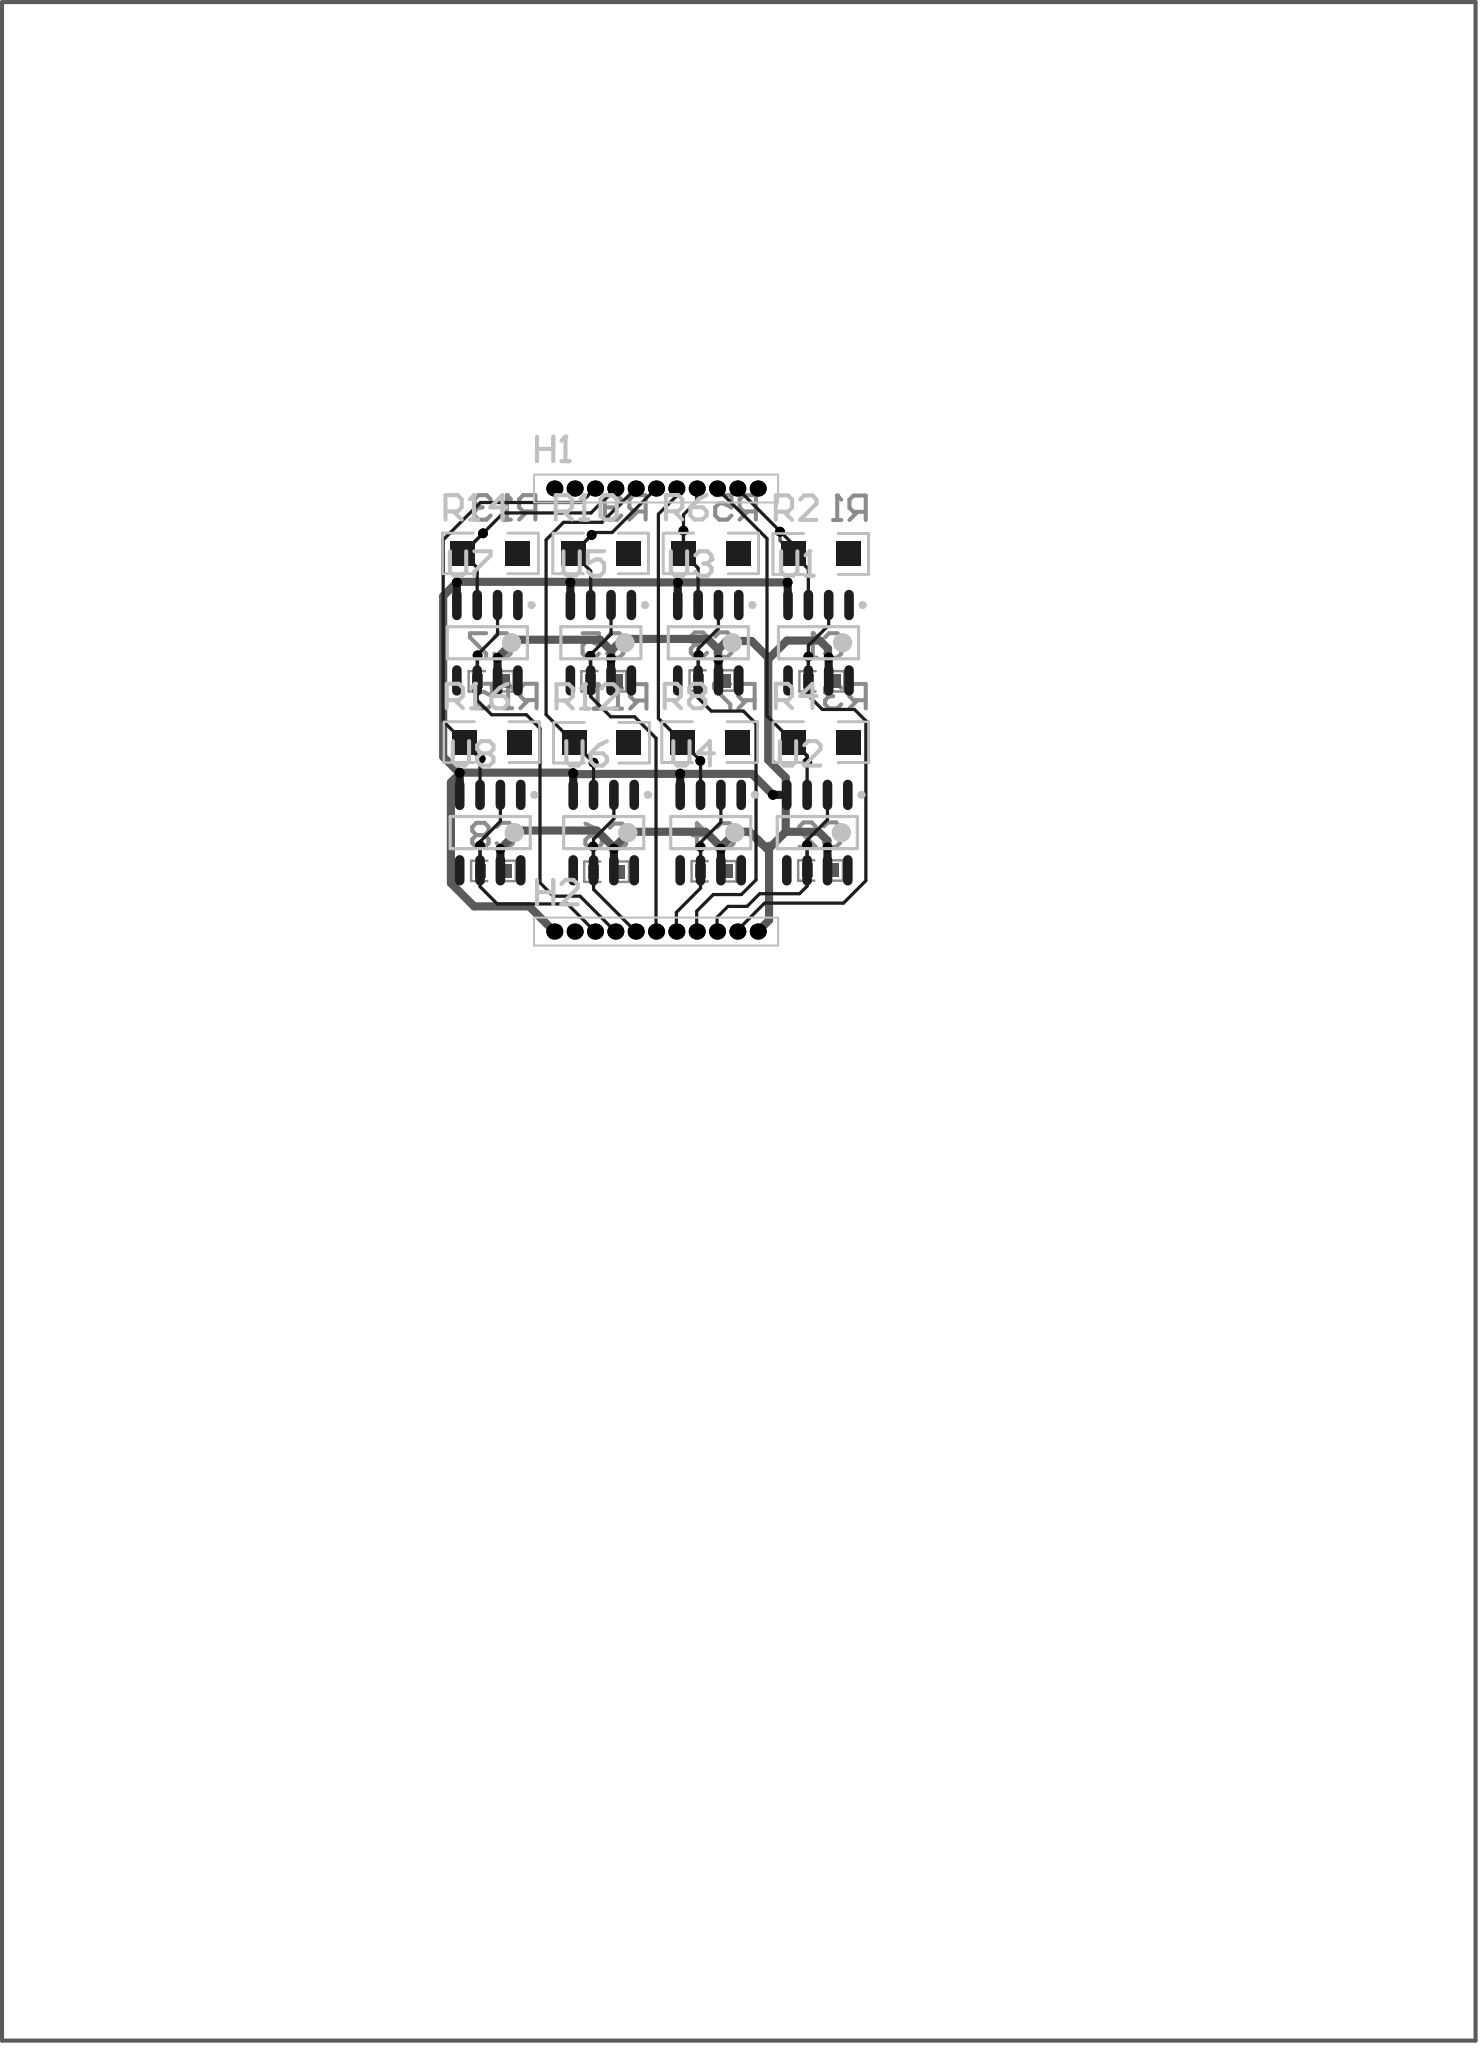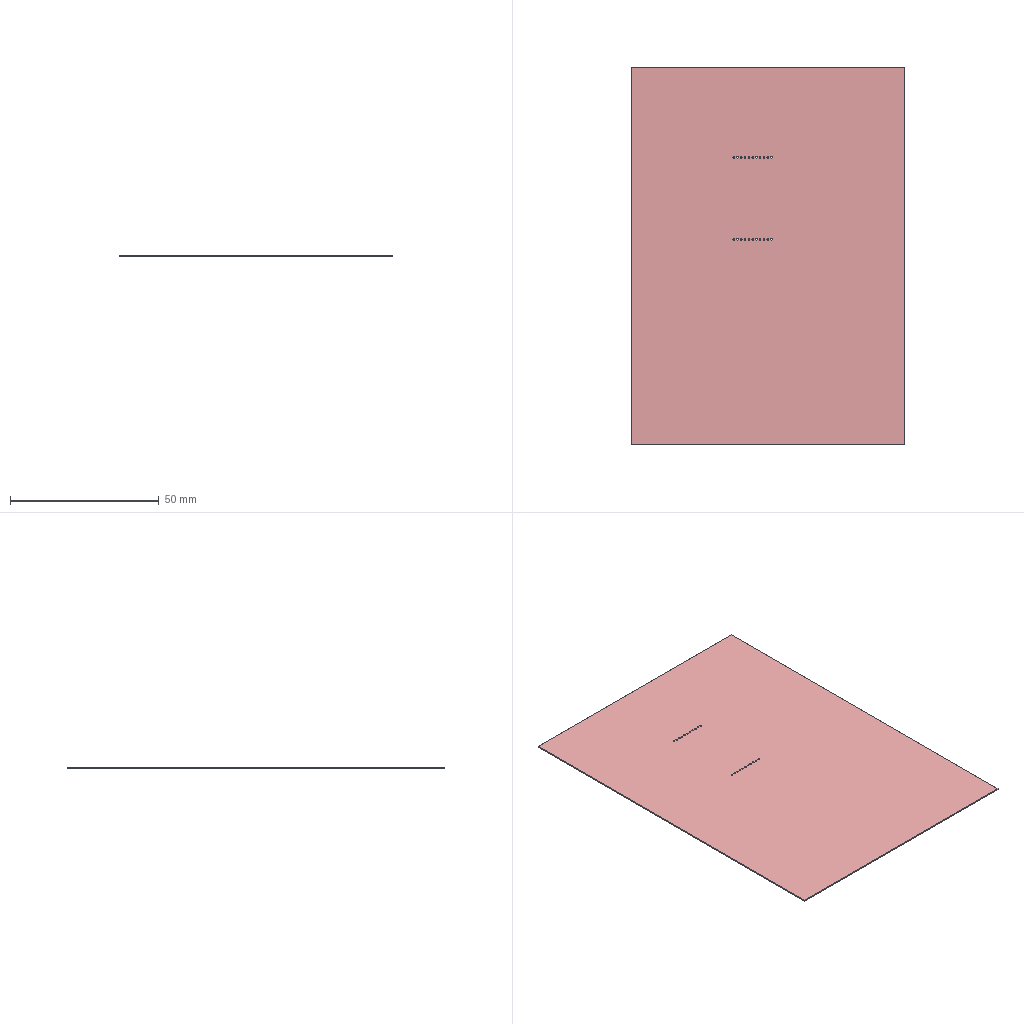Circuit board layout | Altium Designer | box 92 x 127 x 0.4 mm
Layer stack:
# Altium Designer layer stack of  (unit mm; dielectric type: 0 none, 1 core, 2 prepreg, 3 surface material)
index,name,kind,layer,copper_thickness_mm,dielectric_type,dielectric_thickness_mm,dielectric_material,dielectric_constant
0,Top Paste,other,,,,,,
1,Top Overlay,other,,,,,,
2,Top Solder,dielectric,,,3,0.0102,Solder Resist,3.5
3,Top Layer,copper,Top Layer,0.0356,,,,
4,Dielectric1,dielectric,,,0,0.32,FR-4,4.8
5,Bottom Layer,copper,Bottom Layer,0.0356,,,,
6,Bottom Solder,dielectric,,,3,0.0102,Solder Resist,3.5
7,Bottom Overlay,other,,,,,,
8,Bottom Paste,other,,,,,,
# drill layer pairs: low layer,high layer
drill_pair,Top Layer,Bottom Layer
Part placement:
Designator,Comment,Layer,Footprint,Center-X(mm),Center-Y(mm),Rotation
U8,TL061D,TopLayer,TL061_SOIC8,3.648,7.366,270
U7,TL061D,TopLayer,TL061_SOIC8,3.47,19.193,270
U6,TL061D,TopLayer,TL061_SOIC8,10.735,7.366,270
U5,TL061D,TopLayer,TL061_SOIC8,10.557,19.193,270
U4,TL061D,TopLayer,TL061_SOIC8,17.415,7.366,270
U3,TL061D,TopLayer,TL061_SOIC8,17.263,19.193,270
U2,TL061D,TopLayer,TL061_SOIC8,24.07,7.366,270
U1,TL061D,TopLayer,TL061_SOIC8,24.146,19.193,270
R16,1%,TopLayer,1206,3.737,12.995,360
R15,1%,BottomLayer,1206,3.737,12.995,360
R14,1%,TopLayer,1206,3.661,24.756,360
R13,1%,BottomLayer,1206,3.661,24.756,360
R12,1%,TopLayer,1206,10.595,12.97,360
R11,1%,BottomLayer,1206,10.595,12.97,360
R10,1%,TopLayer,1206,10.544,24.756,360
R9,1%,BottomLayer,1206,10.544,24.756,360
R8,1%,TopLayer,1206,17.352,12.995,360
R7,1%,BottomLayer,1206,17.352,12.995,360
R6,1%,TopLayer,1206,17.428,24.756,360
R5,1%,BottomLayer,1206,17.428,24.756,360
R4,1%,TopLayer,1206,24.286,12.995,360
R3,1%,BottomLayer,1206,24.286,12.995,360
R2,1%,TopLayer,1206,24.286,24.73,360
R1,1%,BottomLayer,1206,24.286,24.73,360
H1,Header11,TopLayer,PinHeader11_1.27mm,14,28.8,180
H2,Header11,TopLayer,PinHeader11_1.27mm,14,1.2,180
C8,30pF,BottomLayer,0603,3.851,4.978,180
C7,30pF,BottomLayer,0603,3.699,16.789,180
C6,30pF,BottomLayer,0603,10.913,4.928,180
C5,30pF,BottomLayer,0603,10.735,16.789,180
C4,30pF,BottomLayer,0603,17.618,4.953,180
C3,30pF,BottomLayer,0603,17.491,16.84,180
C2,30pF,BottomLayer,0603,24.273,5.004,180
C1,30pF,BottomLayer,0603,24.349,16.789,180
Pad and via stacks:
# Altium Designer via and pad stacks of  (unit mm). Each distinct definition once, with the count of objects using it.
# via: kind,start_layer,end_layer,hole_mm,diameter_mm,mode(0 simple;1 top-mid-bottom;2 full stack),diameter_per_layer,count,example_net
# pad: kind,layer,hole_mm,hole_type(0 round;1 square;2 slot),plating,top_size,top_shape(1 round;2 rect;3 octagon;9 rounded rect),mid_size,bottom_size,mode,footprint,size_per_layer,count,example
pad,Top Layer,0,0,plated,0.6x1.9,1,0.6x1.9,0.6x1.9,0,TL061_SOIC8,,64,U1.5
pad,Top Layer,0,0,plated,1.524x1.524,2,1.524x1.524,1.524x1.524,0,1206,,16,R2.1
pad,Multi-Layer,0.5334,0,plated,1x1,1,1x1,1x1,0,PinHeader11_1.27mm,,22,H2.8
pad,Bottom Layer,0,0,plated,0.635x0.8128,2,0.635x0.8128,0.635x0.8128,0,0603,,16,C1.2
pad,Bottom Layer,0,0,plated,1.524x1.524,2,1.524x1.524,1.524x1.524,0,1206,,16,R1.1
via,Top Layer,Bottom Layer,0.3048,0.6096,0,,32,-15V
Design rules, without the lines most boards share:
# Altium Designer design rules of  (exported by Altium Designer, unit mm)
# columns: name | kind | enabled | priority | scope1 | scope2 | descriptor | typed fields (field=value)
SilkToSilkClearance | 55 | enabled | 1 | All | All | Silk to Silk (Clearance=0mil) (All),(All) |
SilkscreenOverComponentPads | 54 | enabled | 1 | IsPad | All | Silk To Solder Mask (Clearance=0mil) (IsPad),(All) |
MinimumSolderMaskSliver | 53 | enabled | 1 | All | All | Minimum Solder Mask Sliver (Gap=0mil) (All),(All) |
HoleToHoleClearance | 52 | enabled | 1 | All | All | Hole To Hole Clearance (Gap=10mil) (All),(All) | gap=0.254
DiffPairsRouting | 51 | enabled | 1 | All | All | Differential Pairs Uncoupled Length using the Gap Constraints (Min=10mil) (Max=10mil) (Prefered=10mil)  and Width Constraints (Min=15mil) (Max=15mil) (Prefered=15mil) (All) |
HoleSize | 42 | enabled | 1 | All | All | Hole Size Constraint (Min=11.811mil) (Max=150mil) (All) |
Testpoint | 43 | enabled | 1 | (IsPad And (OnTopLayer Or OnBottomLayer)) | All | Fabrication Testpoint Style (Under Component=Yes) ((IsPad And (OnTopLayer Or OnBottomLayer))) |
TestPointUsage | 44 | enabled | 1 | All | All | Fabrication Testpoint Usage (Valid =One Required, Allow multiple per net=No) (All) |
SolderMaskExpansion | 13 | enabled | 1 | All | All | Solder Mask Expansion (Expansion =4mil) (All) | expansion=0.1016
PasteMaskExpansion | 14 | enabled | 1 | All | All | Paste Mask Expansion (Expansion =0mil) (All) | expansion=0
RoutingVias | 11 | enabled | 1 | All | All | Routing Via (MinHoleWidth=12mil) (MaxHoleWidth=12mil) (PreferredHoleWidth=12mil) (MinWidth=24mil) (MaxWidth=24mil) (PreferedWidth=24mil) (All) | via_min_hole=0.3048 via_max_hole=0.3048 via_preferred_diameter=0.6096 via_preferred_hole=0.3048
Width | 2 | enabled | 1 | All | All | Width Constraint (Min=8mil) (Max=20mil) (Preferred=8mil) (All) |
PolygonConnect | 20 | enabled | 1 | All | All | Polygon Connect Rule(Relief Connect )(Conductor Width=10mil) (Relief Angle=90 Angle) (Entries=4) (Air Gap Width=10mil) (All),(All) | connect_style(0=relief,1=direct,2=none)=0 relief_conductor_width=0.254 relief_entries=4
PlaneConnect | 6 | enabled | 1 | All | All | Power Plane Connect Rule(Relief Connect )(Expansion=20mil) (Conductor Width=10mil) (Air Gap=10mil) (Entries=4) (All) | relief_conductor_width=0.254 relief_entries=4 relief_expansion=0.508
Clearance | 0 | enabled | 1 | All | All | Clearance Constraint (Gap=6mil) (All),(All) | gap=0.1524